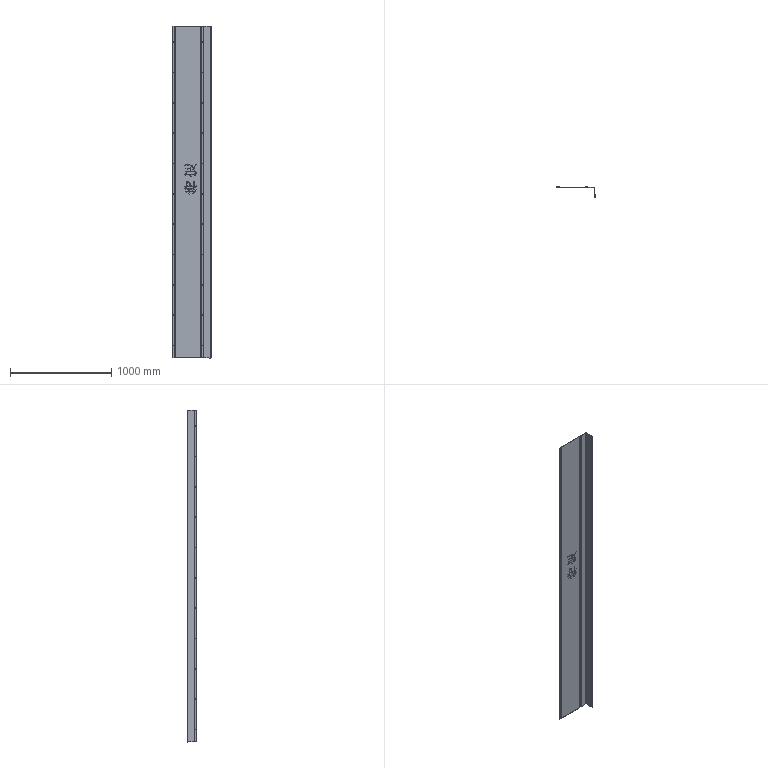Part | STEP file | TS-S97 TBD | 1 solid | 254 faces | box 375.999 x 97.999 x 3283 mm | volume 1855793 mm3 | plane 136 | cylinder 85 | spline 33 | commonest cylinder face diameters 5.4 x66 0.4 x9 2.8 x9 10 x1